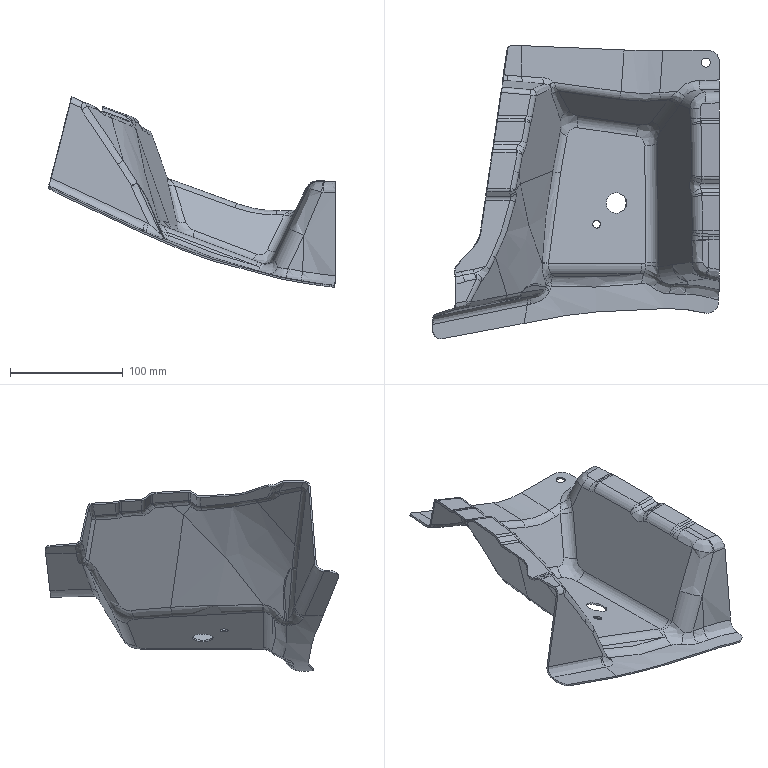Part | 1 solid | 386 faces | box 255.436 x 260.625 x 168.935 mm | volume 122902 mm3 | spline 271 | cylinder 78 | plane 33 | other 4 | commonest cylinder face diameters 10 x11 17 x7 20 x7 7 x6 13 x5 18 x3